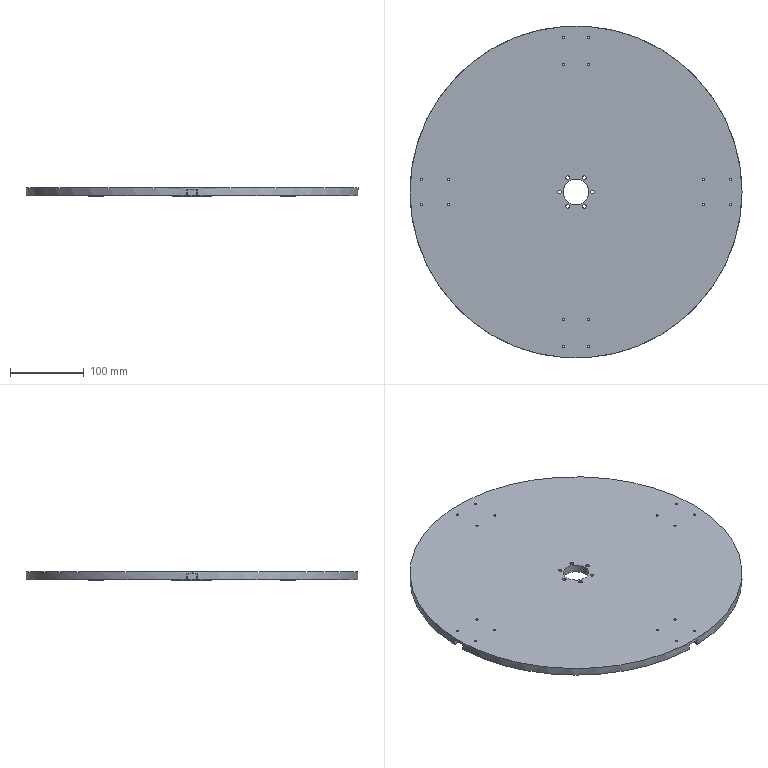Part | STEP file | Indexing plate | 1 solid | 437 faces | box 450 x 450 x 12 mm | volume 1702254 mm3 | plane 234 | spline 115 | cylinder 88 | commonest cylinder face diameters 2.9 x32 6.5 x32 5 x12 4 x8 35 x2 450 x2